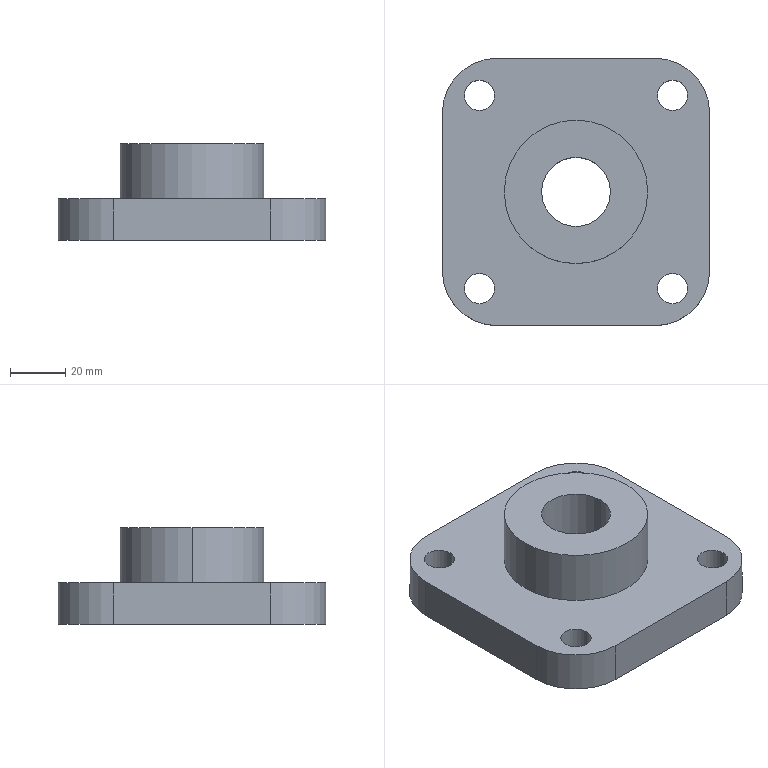Part | STEP file | Bearing housing 1 | 1 solid | 23 faces | box 97 x 97 x 35 mm | volume 155576 mm3 | cylinder 16 | plane 7 | commonest cylinder face diameters 11 x8 40 x4 25 x2 52 x2
STEP:
#1=CARTESIAN_POINT('',(28.236,16.5,35.));
#2=VERTEX_POINT('',#1);
#3=CARTESIAN_POINT('',(3.236,16.5,35.));
#4=VERTEX_POINT('',#3);
#5=CARTESIAN_POINT('',(15.736,16.5,35.));
#6=DIRECTION('',(0.,0.,-1.));
#7=DIRECTION('',(-1.,0.,0.));
#8=AXIS2_PLACEMENT_3D('',#5,#6,#7);
#9=CIRCLE('',#8,12.5);
#10=EDGE_CURVE('',#2,#4,#9,.T.);
#11=ORIENTED_EDGE('',*,*,#10,.F.);
#12=CARTESIAN_POINT('',(28.236,16.5,0.));
#13=VERTEX_POINT('',#12);
#14=CARTESIAN_POINT('',(28.236,16.5,15.));
#15=DIRECTION('',(0.,0.,-1.));
#16=VECTOR('',#15,1000.);
#17=LINE('',#14,#16);
#18=EDGE_CURVE('',#2,#13,#17,.T.);
#19=ORIENTED_EDGE('',*,*,#18,.T.);
#20=CARTESIAN_POINT('',(3.236,16.5,0.));
#21=VERTEX_POINT('',#20);
#22=CARTESIAN_POINT('',(15.736,16.5,0.));
#23=DIRECTION('',(0.,0.,-1.));
#24=DIRECTION('',(-1.,0.,0.));
#25=AXIS2_PLACEMENT_3D('',#22,#23,#24);
#26=CIRCLE('',#25,12.5);
#27=EDGE_CURVE('',#13,#21,#26,.T.);
#28=ORIENTED_EDGE('',*,*,#27,.T.);
#29=CARTESIAN_POINT('',(3.236,16.5,15.));
#30=DIRECTION('',(0.,0.,-1.));
#31=VECTOR('',#30,1000.);
#32=LINE('',#29,#31);
#33=EDGE_CURVE('',#4,#21,#32,.T.);
#34=ORIENTED_EDGE('',*,*,#33,.F.);
#35=EDGE_LOOP('',(#11,#19,#28,#34));
#36=FACE_OUTER_BOUND('',#35,.T.);
#37=CARTESIAN_POINT('',(15.736,16.5,15.));
#38=DIRECTION('',(0.,0.,-1.));
#39=DIRECTION('',(-1.,0.,0.));
#40=AXIS2_PLACEMENT_3D('',#37,#38,#39);
#41=CYLINDRICAL_SURFACE('',#40,12.5);
#42=ADVANCED_FACE('',(#36),#41,.F.);
#43=CARTESIAN_POINT('',(56.236,-18.5,15.));
#44=VERTEX_POINT('',#43);
#45=CARTESIAN_POINT('',(45.236,-18.5,15.));
#46=VERTEX_POINT('',#45);
#47=CARTESIAN_POINT('',(50.736,-18.5,15.));
#48=DIRECTION('',(0.,0.,-1.));
#49=DIRECTION('',(-1.,0.,0.));
#50=AXIS2_PLACEMENT_3D('',#47,#48,#49);
#51=CIRCLE('',#50,5.5);
#52=EDGE_CURVE('',#44,#46,#51,.T.);
#53=ORIENTED_EDGE('',*,*,#52,.F.);
#54=CARTESIAN_POINT('',(56.236,-18.5,0.));
#55=VERTEX_POINT('',#54);
#56=CARTESIAN_POINT('',(56.236,-18.5,15.));
#57=DIRECTION('',(0.,0.,-1.));
#58=VECTOR('',#57,1000.);
#59=LINE('',#56,#58);
#60=EDGE_CURVE('',#44,#55,#59,.T.);
#61=ORIENTED_EDGE('',*,*,#60,.T.);
#62=CARTESIAN_POINT('',(45.236,-18.5,0.));
#63=VERTEX_POINT('',#62);
#64=CARTESIAN_POINT('',(50.736,-18.5,0.));
#65=DIRECTION('',(0.,0.,-1.));
#66=DIRECTION('',(-1.,0.,0.));
#67=AXIS2_PLACEMENT_3D('',#64,#65,#66);
#68=CIRCLE('',#67,5.5);
#69=EDGE_CURVE('',#55,#63,#68,.T.);
#70=ORIENTED_EDGE('',*,*,#69,.T.);
#71=CARTESIAN_POINT('',(45.236,-18.5,15.));
#72=DIRECTION('',(0.,0.,-1.));
#73=VECTOR('',#72,1000.);
#74=LINE('',#71,#73);
#75=EDGE_CURVE('',#46,#63,#74,.T.);
#76=ORIENTED_EDGE('',*,*,#75,.F.);
#77=EDGE_LOOP('',(#53,#61,#70,#76));
#78=FACE_OUTER_BOUND('',#77,.T.);
#79=CARTESIAN_POINT('',(50.736,-18.5,15.));
#80=DIRECTION('',(0.,0.,-1.));
#81=DIRECTION('',(-1.,0.,0.));
#82=AXIS2_PLACEMENT_3D('',#79,#80,#81);
#83=CYLINDRICAL_SURFACE('',#82,5.5);
#84=ADVANCED_FACE('',(#78),#83,.F.);
#85=CARTESIAN_POINT('',(-13.764,51.5,15.));
#86=VERTEX_POINT('',#85);
#87=CARTESIAN_POINT('',(-24.764,51.5,15.));
#88=VERTEX_POINT('',#87);
#89=CARTESIAN_POINT('',(-19.264,51.5,15.));
#90=DIRECTION('',(0.,0.,-1.));
#91=DIRECTION('',(-1.,0.,0.));
#92=AXIS2_PLACEMENT_3D('',#89,#90,#91);
#93=CIRCLE('',#92,5.5);
#94=EDGE_CURVE('',#86,#88,#93,.T.);
#95=ORIENTED_EDGE('',*,*,#94,.F.);
#96=CARTESIAN_POINT('',(-13.764,51.5,0.));
#97=VERTEX_POINT('',#96);
#98=CARTESIAN_POINT('',(-13.764,51.5,15.));
#99=DIRECTION('',(0.,0.,-1.));
#100=VECTOR('',#99,1000.);
#101=LINE('',#98,#100);
#102=EDGE_CURVE('',#86,#97,#101,.T.);
#103=ORIENTED_EDGE('',*,*,#102,.T.);
#104=CARTESIAN_POINT('',(-24.764,51.5,0.));
#105=VERTEX_POINT('',#104);
#106=CARTESIAN_POINT('',(-19.264,51.5,0.));
#107=DIRECTION('',(0.,0.,-1.));
#108=DIRECTION('',(-1.,0.,0.));
#109=AXIS2_PLACEMENT_3D('',#106,#107,#108);
#110=CIRCLE('',#109,5.5);
#111=EDGE_CURVE('',#97,#105,#110,.T.);
#112=ORIENTED_EDGE('',*,*,#111,.T.);
#113=CARTESIAN_POINT('',(-24.764,51.5,15.));
#114=DIRECTION('',(0.,0.,-1.));
#115=VECTOR('',#114,1000.);
#116=LINE('',#113,#115);
#117=EDGE_CURVE('',#88,#105,#116,.T.);
#118=ORIENTED_EDGE('',*,*,#117,.F.);
#119=EDGE_LOOP('',(#95,#103,#112,#118));
#120=FACE_OUTER_BOUND('',#119,.T.);
#121=CARTESIAN_POINT('',(-19.264,51.5,15.));
#122=DIRECTION('',(0.,0.,-1.));
#123=DIRECTION('',(-1.,0.,0.));
#124=AXIS2_PLACEMENT_3D('',#121,#122,#123);
#125=CYLINDRICAL_SURFACE('',#124,5.5);
#126=ADVANCED_FACE('',(#120),#125,.F.);
#127=CARTESIAN_POINT('',(56.236,51.5,15.));
#128=VERTEX_POINT('',#127);
#129=CARTESIAN_POINT('',(45.236,51.5,15.));
#130=VERTEX_POINT('',#129);
#131=CARTESIAN_POINT('',(50.736,51.5,15.));
#132=DIRECTION('',(0.,0.,-1.));
#133=DIRECTION('',(-1.,0.,0.));
#134=AXIS2_PLACEMENT_3D('',#131,#132,#133);
#135=CIRCLE('',#134,5.5);
#136=EDGE_CURVE('',#128,#130,#135,.T.);
#137=ORIENTED_EDGE('',*,*,#136,.F.);
#138=CARTESIAN_POINT('',(56.236,51.5,0.));
#139=VERTEX_POINT('',#138);
#140=CARTESIAN_POINT('',(56.236,51.5,15.));
#141=DIRECTION('',(0.,0.,-1.));
#142=VECTOR('',#141,1000.);
#143=LINE('',#140,#142);
#144=EDGE_CURVE('',#128,#139,#143,.T.);
#145=ORIENTED_EDGE('',*,*,#144,.T.);
#146=CARTESIAN_POINT('',(45.236,51.5,0.));
#147=VERTEX_POINT('',#146);
#148=CARTESIAN_POINT('',(50.736,51.5,0.));
#149=DIRECTION('',(0.,0.,-1.));
#150=DIRECTION('',(-1.,0.,0.));
#151=AXIS2_PLACEMENT_3D('',#148,#149,#150);
#152=CIRCLE('',#151,5.5);
#153=EDGE_CURVE('',#139,#147,#152,.T.);
#154=ORIENTED_EDGE('',*,*,#153,.T.);
#155=CARTESIAN_POINT('',(45.236,51.5,15.));
#156=DIRECTION('',(0.,0.,-1.));
#157=VECTOR('',#156,1000.);
#158=LINE('',#155,#157);
#159=EDGE_CURVE('',#130,#147,#158,.T.);
#160=ORIENTED_EDGE('',*,*,#159,.F.);
#161=EDGE_LOOP('',(#137,#145,#154,#160));
#162=FACE_OUTER_BOUND('',#161,.T.);
#163=CARTESIAN_POINT('',(50.736,51.5,15.));
#164=DIRECTION('',(0.,0.,-1.));
#165=DIRECTION('',(-1.,0.,0.));
#166=AXIS2_PLACEMENT_3D('',#163,#164,#165);
#167=CYLINDRICAL_SURFACE('',#166,5.5);
#168=ADVANCED_FACE('',(#162),#167,.F.);
#169=CARTESIAN_POINT('',(-13.764,-18.5,15.));
#170=VERTEX_POINT('',#169);
#171=CARTESIAN_POINT('',(-24.764,-18.5,15.));
#172=VERTEX_POINT('',#171);
#173=CARTESIAN_POINT('',(-19.264,-18.5,15.));
#174=DIRECTION('',(0.,0.,-1.));
#175=DIRECTION('',(-1.,0.,0.));
#176=AXIS2_PLACEMENT_3D('',#173,#174,#175);
#177=CIRCLE('',#176,5.5);
#178=EDGE_CURVE('',#170,#172,#177,.T.);
#179=ORIENTED_EDGE('',*,*,#178,.F.);
#180=CARTESIAN_POINT('',(-13.764,-18.5,0.));
#181=VERTEX_POINT('',#180);
#182=CARTESIAN_POINT('',(-13.764,-18.5,15.));
#183=DIRECTION('',(0.,0.,-1.));
#184=VECTOR('',#183,1000.);
#185=LINE('',#182,#184);
#186=EDGE_CURVE('',#170,#181,#185,.T.);
#187=ORIENTED_EDGE('',*,*,#186,.T.);
#188=CARTESIAN_POINT('',(-24.764,-18.5,0.));
#189=VERTEX_POINT('',#188);
#190=CARTESIAN_POINT('',(-19.264,-18.5,0.));
#191=DIRECTION('',(0.,0.,-1.));
#192=DIRECTION('',(-1.,0.,0.));
#193=AXIS2_PLACEMENT_3D('',#190,#191,#192);
#194=CIRCLE('',#193,5.5);
#195=EDGE_CURVE('',#181,#189,#194,.T.);
#196=ORIENTED_EDGE('',*,*,#195,.T.);
#197=CARTESIAN_POINT('',(-24.764,-18.5,15.));
#198=DIRECTION('',(0.,0.,-1.));
#199=VECTOR('',#198,1000.);
#200=LINE('',#197,#199);
#201=EDGE_CURVE('',#172,#189,#200,.T.);
#202=ORIENTED_EDGE('',*,*,#201,.F.);
#203=EDGE_LOOP('',(#179,#187,#196,#202));
#204=FACE_OUTER_BOUND('',#203,.T.);
#205=CARTESIAN_POINT('',(-19.264,-18.5,15.));
#206=DIRECTION('',(0.,0.,-1.));
#207=DIRECTION('',(-1.,0.,0.));
#208=AXIS2_PLACEMENT_3D('',#205,#206,#207);
#209=CYLINDRICAL_SURFACE('',#208,5.5);
#210=ADVANCED_FACE('',(#204),#209,.F.);
#211=CARTESIAN_POINT('',(41.736,16.5,35.));
#212=VERTEX_POINT('',#211);
#213=CARTESIAN_POINT('',(-10.264,16.5,35.));
#214=VERTEX_POINT('',#213);
#215=CARTESIAN_POINT('',(15.736,16.5,35.));
#216=DIRECTION('',(0.,0.,1.));
#217=DIRECTION('',(-1.,0.,0.));
#218=AXIS2_PLACEMENT_3D('',#215,#216,#217);
#219=CIRCLE('',#218,26.);
#220=EDGE_CURVE('',#212,#214,#219,.T.);
#221=ORIENTED_EDGE('',*,*,#220,.F.);
#222=CARTESIAN_POINT('',(41.736,16.5,15.));
#223=VERTEX_POINT('',#222);
#224=CARTESIAN_POINT('',(41.736,16.5,35.));
#225=DIRECTION('',(0.,0.,-1.));
#226=VECTOR('',#225,1000.);
#227=LINE('',#224,#226);
#228=EDGE_CURVE('',#212,#223,#227,.T.);
#229=ORIENTED_EDGE('',*,*,#228,.T.);
#230=CARTESIAN_POINT('',(-10.264,16.5,15.));
#231=VERTEX_POINT('',#230);
#232=CARTESIAN_POINT('',(15.736,16.5,15.));
#233=DIRECTION('',(0.,0.,-1.));
#234=DIRECTION('',(-1.,0.,0.));
#235=AXIS2_PLACEMENT_3D('',#232,#233,#234);
#236=CIRCLE('',#235,26.);
#237=EDGE_CURVE('',#231,#223,#236,.T.);
#238=ORIENTED_EDGE('',*,*,#237,.F.);
#239=CARTESIAN_POINT('',(-10.264,16.5,35.));
#240=DIRECTION('',(0.,0.,-1.));
#241=VECTOR('',#240,1000.);
#242=LINE('',#239,#241);
#243=EDGE_CURVE('',#214,#231,#242,.T.);
#244=ORIENTED_EDGE('',*,*,#243,.F.);
#245=EDGE_LOOP('',(#221,#229,#238,#244));
#246=FACE_OUTER_BOUND('',#245,.T.);
#247=CARTESIAN_POINT('',(15.736,16.5,35.));
#248=DIRECTION('',(0.,0.,-1.));
#249=DIRECTION('',(-1.,0.,0.));
#250=AXIS2_PLACEMENT_3D('',#247,#248,#249);
#251=CYLINDRICAL_SURFACE('',#250,26.);
#252=ADVANCED_FACE('',(#246),#251,.T.);
#253=CARTESIAN_POINT('',(15.736,16.5,0.));
#254=DIRECTION('',(0.,0.,-1.));
#255=DIRECTION('',(-1.,0.,0.));
#256=AXIS2_PLACEMENT_3D('',#253,#254,#255);
#257=CIRCLE('',#256,12.5);
#258=EDGE_CURVE('',#21,#13,#257,.T.);
#259=ORIENTED_EDGE('',*,*,#258,.F.);
#260=ORIENTED_EDGE('',*,*,#27,.F.);
#261=EDGE_LOOP('',(#259,#260));
#262=FACE_BOUND('',#261,.T.);
#263=CARTESIAN_POINT('',(50.736,-18.5,0.));
#264=DIRECTION('',(0.,0.,-1.));
#265=DIRECTION('',(-1.,0.,0.));
#266=AXIS2_PLACEMENT_3D('',#263,#264,#265);
#267=CIRCLE('',#266,5.5);
#268=EDGE_CURVE('',#63,#55,#267,.T.);
#269=ORIENTED_EDGE('',*,*,#268,.F.);
#270=ORIENTED_EDGE('',*,*,#69,.F.);
#271=EDGE_LOOP('',(#269,#270));
#272=FACE_BOUND('',#271,.T.);
#273=CARTESIAN_POINT('',(-19.264,51.5,0.));
#274=DIRECTION('',(0.,0.,-1.));
#275=DIRECTION('',(-1.,0.,0.));
#276=AXIS2_PLACEMENT_3D('',#273,#274,#275);
#277=CIRCLE('',#276,5.5);
#278=EDGE_CURVE('',#105,#97,#277,.T.);
#279=ORIENTED_EDGE('',*,*,#278,.F.);
#280=ORIENTED_EDGE('',*,*,#111,.F.);
#281=EDGE_LOOP('',(#279,#280));
#282=FACE_BOUND('',#281,.T.);
#283=CARTESIAN_POINT('',(-32.764,-12.,0.));
#284=VERTEX_POINT('',#283);
#285=CARTESIAN_POINT('',(-12.764,-32.,0.));
#286=VERTEX_POINT('',#285);
#287=CARTESIAN_POINT('',(-12.764,-12.,0.));
#288=DIRECTION('',(0.,0.,1.));
#289=DIRECTION('',(-1.,0.,0.));
#290=AXIS2_PLACEMENT_3D('',#287,#288,#289);
#291=CIRCLE('',#290,20.);
#292=EDGE_CURVE('',#284,#286,#291,.T.);
#293=ORIENTED_EDGE('',*,*,#292,.F.);
#294=CARTESIAN_POINT('',(-32.764,45.,0.));
#295=VERTEX_POINT('',#294);
#296=CARTESIAN_POINT('',(-32.764,65.,0.));
#297=DIRECTION('',(0.,-1.,0.));
#298=VECTOR('',#297,1000.);
#299=LINE('',#296,#298);
#300=EDGE_CURVE('',#295,#284,#299,.T.);
#301=ORIENTED_EDGE('',*,*,#300,.F.);
#302=CARTESIAN_POINT('',(-12.764,65.,0.));
#303=VERTEX_POINT('',#302);
#304=CARTESIAN_POINT('',(-12.764,45.,0.));
#305=DIRECTION('',(0.,0.,1.));
#306=DIRECTION('',(-1.,0.,0.));
#307=AXIS2_PLACEMENT_3D('',#304,#305,#306);
#308=CIRCLE('',#307,20.);
#309=EDGE_CURVE('',#303,#295,#308,.T.);
#310=ORIENTED_EDGE('',*,*,#309,.F.);
#311=CARTESIAN_POINT('',(44.236,65.,0.));
#312=VERTEX_POINT('',#311);
#313=CARTESIAN_POINT('',(-32.764,65.,0.));
#314=DIRECTION('',(-1.,0.,0.));
#315=VECTOR('',#314,1000.);
#316=LINE('',#313,#315);
#317=EDGE_CURVE('',#312,#303,#316,.T.);
#318=ORIENTED_EDGE('',*,*,#317,.F.);
#319=CARTESIAN_POINT('',(64.236,45.,0.));
#320=VERTEX_POINT('',#319);
#321=CARTESIAN_POINT('',(44.236,45.,0.));
#322=DIRECTION('',(0.,0.,1.));
#323=DIRECTION('',(-1.,0.,0.));
#324=AXIS2_PLACEMENT_3D('',#321,#322,#323);
#325=CIRCLE('',#324,20.);
#326=EDGE_CURVE('',#320,#312,#325,.T.);
#327=ORIENTED_EDGE('',*,*,#326,.F.);
#328=CARTESIAN_POINT('',(64.236,-12.,0.));
#329=VERTEX_POINT('',#328);
#330=CARTESIAN_POINT('',(64.236,65.,0.));
#331=DIRECTION('',(0.,1.,0.));
#332=VECTOR('',#331,1000.);
#333=LINE('',#330,#332);
#334=EDGE_CURVE('',#329,#320,#333,.T.);
#335=ORIENTED_EDGE('',*,*,#334,.F.);
#336=CARTESIAN_POINT('',(44.236,-32.,0.));
#337=VERTEX_POINT('',#336);
#338=CARTESIAN_POINT('',(44.236,-12.,0.));
#339=DIRECTION('',(0.,0.,1.));
#340=DIRECTION('',(-1.,0.,0.));
#341=AXIS2_PLACEMENT_3D('',#338,#339,#340);
#342=CIRCLE('',#341,20.);
#343=EDGE_CURVE('',#337,#329,#342,.T.);
#344=ORIENTED_EDGE('',*,*,#343,.F.);
#345=CARTESIAN_POINT('',(-32.764,-32.,0.));
#346=DIRECTION('',(1.,0.,0.));
#347=VECTOR('',#346,1000.);
#348=LINE('',#345,#347);
#349=EDGE_CURVE('',#286,#337,#348,.T.);
#350=ORIENTED_EDGE('',*,*,#349,.F.);
#351=EDGE_LOOP('',(#293,#301,#310,#318,#327,#335,#344,#350));
#352=FACE_OUTER_BOUND('',#351,.T.);
#353=CARTESIAN_POINT('',(50.736,51.5,0.));
#354=DIRECTION('',(0.,0.,-1.));
#355=DIRECTION('',(-1.,0.,0.));
#356=AXIS2_PLACEMENT_3D('',#353,#354,#355);
#357=CIRCLE('',#356,5.5);
#358=EDGE_CURVE('',#147,#139,#357,.T.);
#359=ORIENTED_EDGE('',*,*,#358,.F.);
#360=ORIENTED_EDGE('',*,*,#153,.F.);
#361=EDGE_LOOP('',(#359,#360));
#362=FACE_BOUND('',#361,.T.);
#363=CARTESIAN_POINT('',(-19.264,-18.5,0.));
#364=DIRECTION('',(0.,0.,-1.));
#365=DIRECTION('',(-1.,0.,0.));
#366=AXIS2_PLACEMENT_3D('',#363,#364,#365);
#367=CIRCLE('',#366,5.5);
#368=EDGE_CURVE('',#189,#181,#367,.T.);
#369=ORIENTED_EDGE('',*,*,#368,.F.);
#370=ORIENTED_EDGE('',*,*,#195,.F.);
#371=EDGE_LOOP('',(#369,#370));
#372=FACE_BOUND('',#371,.T.);
#373=CARTESIAN_POINT('',(-32.764,65.,0.));
#374=DIRECTION('',(0.,0.,1.));
#375=DIRECTION('',(1.,0.,0.));
#376=AXIS2_PLACEMENT_3D('',#373,#374,#375);
#377=PLANE('',#376);
#378=ADVANCED_FACE('',(#262,#272,#282,#352,#362,#372),#377,.F.);
#379=ORIENTED_EDGE('',*,*,#18,.F.);
#380=CARTESIAN_POINT('',(15.736,16.5,35.));
#381=DIRECTION('',(0.,0.,-1.));
#382=DIRECTION('',(-1.,0.,0.));
#383=AXIS2_PLACEMENT_3D('',#380,#381,#382);
#384=CIRCLE('',#383,12.5);
#385=EDGE_CURVE('',#4,#2,#384,.T.);
#386=ORIENTED_EDGE('',*,*,#385,.F.);
#387=ORIENTED_EDGE('',*,*,#33,.T.);
#388=ORIENTED_EDGE('',*,*,#258,.T.);
#389=EDGE_LOOP('',(#379,#386,#387,#388));
#390=FACE_OUTER_BOUND('',#389,.T.);
#391=CARTESIAN_POINT('',(15.736,16.5,15.));
#392=DIRECTION('',(0.,0.,-1.));
#393=DIRECTION('',(-1.,0.,0.));
#394=AXIS2_PLACEMENT_3D('',#391,#392,#393);
#395=CYLINDRICAL_SURFACE('',#394,12.5);
#396=ADVANCED_FACE('',(#390),#395,.F.);
#397=ORIENTED_EDGE('',*,*,#60,.F.);
#398=CARTESIAN_POINT('',(50.736,-18.5,15.));
#399=DIRECTION('',(0.,0.,-1.));
#400=DIRECTION('',(-1.,0.,0.));
#401=AXIS2_PLACEMENT_3D('',#398,#399,#400);
#402=CIRCLE('',#401,5.5);
#403=EDGE_CURVE('',#46,#44,#402,.T.);
#404=ORIENTED_EDGE('',*,*,#403,.F.);
#405=ORIENTED_EDGE('',*,*,#75,.T.);
#406=ORIENTED_EDGE('',*,*,#268,.T.);
#407=EDGE_LOOP('',(#397,#404,#405,#406));
#408=FACE_OUTER_BOUND('',#407,.T.);
#409=CARTESIAN_POINT('',(50.736,-18.5,15.));
#410=DIRECTION('',(0.,0.,-1.));
#411=DIRECTION('',(-1.,0.,0.));
#412=AXIS2_PLACEMENT_3D('',#409,#410,#411);
#413=CYLINDRICAL_SURFACE('',#412,5.5);
#414=ADVANCED_FACE('',(#408),#413,.F.);
#415=ORIENTED_EDGE('',*,*,#102,.F.);
#416=CARTESIAN_POINT('',(-19.264,51.5,15.));
#417=DIRECTION('',(0.,0.,-1.));
#418=DIRECTION('',(-1.,0.,0.));
#419=AXIS2_PLACEMENT_3D('',#416,#417,#418);
#420=CIRCLE('',#419,5.5);
#421=EDGE_CURVE('',#88,#86,#420,.T.);
#422=ORIENTED_EDGE('',*,*,#421,.F.);
#423=ORIENTED_EDGE('',*,*,#117,.T.);
#424=ORIENTED_EDGE('',*,*,#278,.T.);
#425=EDGE_LOOP('',(#415,#422,#423,#424));
#426=FACE_OUTER_BOUND('',#425,.T.);
#427=CARTESIAN_POINT('',(-19.264,51.5,15.));
#428=DIRECTION('',(0.,0.,-1.));
#429=DIRECTION('',(-1.,0.,0.));
#430=AXIS2_PLACEMENT_3D('',#427,#428,#429);
#431=CYLINDRICAL_SURFACE('',#430,5.5);
#432=ADVANCED_FACE('',(#426),#431,.F.);
#433=CARTESIAN_POINT('',(-12.764,-32.,15.));
#434=VERTEX_POINT('',#433);
#435=CARTESIAN_POINT('',(-12.764,-32.,15.));
#436=DIRECTION('',(0.,0.,1.));
#437=VECTOR('',#436,1000.);
#438=LINE('',#435,#437);
#439=EDGE_CURVE('',#286,#434,#438,.T.);
#440=ORIENTED_EDGE('',*,*,#439,.F.);
#441=ORIENTED_EDGE('',*,*,#349,.T.);
#442=CARTESIAN_POINT('',(44.236,-32.,15.));
#443=VERTEX_POINT('',#442);
#444=CARTESIAN_POINT('',(44.236,-32.,15.));
#445=DIRECTION('',(0.,0.,-1.));
#446=VECTOR('',#445,1000.);
#447=LINE('',#444,#446);
#448=EDGE_CURVE('',#443,#337,#447,.T.);
#449=ORIENTED_EDGE('',*,*,#448,.F.);
#450=CARTESIAN_POINT('',(-32.764,-32.,15.));
#451=DIRECTION('',(1.,0.,0.));
#452=VECTOR('',#451,1000.);
#453=LINE('',#450,#452);
#454=EDGE_CURVE('',#434,#443,#453,.T.);
#455=ORIENTED_EDGE('',*,*,#454,.F.);
#456=EDGE_LOOP('',(#440,#441,#449,#455));
#457=FACE_OUTER_BOUND('',#456,.T.);
#458=CARTESIAN_POINT('',(-32.764,-32.,15.));
#459=DIRECTION('',(0.,1.,0.));
#460=DIRECTION('',(0.,0.,1.));
#461=AXIS2_PLACEMENT_3D('',#458,#459,#460);
#462=PLANE('',#461);
#463=ADVANCED_FACE('',(#457),#462,.F.);
#464=ORIENTED_EDGE('',*,*,#292,.T.);
#465=ORIENTED_EDGE('',*,*,#439,.T.);
#466=CARTESIAN_POINT('',(-32.764,-12.,15.));
#467=VERTEX_POINT('',#466);
#468=CARTESIAN_POINT('',(-12.764,-12.,15.));
#469=DIRECTION('',(0.,0.,-1.));
#470=DIRECTION('',(-1.,0.,0.));
#471=AXIS2_PLACEMENT_3D('',#468,#469,#470);
#472=CIRCLE('',#471,20.);
#473=EDGE_CURVE('',#434,#467,#472,.T.);
#474=ORIENTED_EDGE('',*,*,#473,.T.);
#475=CARTESIAN_POINT('',(-32.764,-12.,15.));
#476=DIRECTION('',(0.,0.,-1.));
#477=VECTOR('',#476,1000.);
#478=LINE('',#475,#477);
#479=EDGE_CURVE('',#467,#284,#478,.T.);
#480=ORIENTED_EDGE('',*,*,#479,.T.);
#481=EDGE_LOOP('',(#464,#465,#474,#480));
#482=FACE_OUTER_BOUND('',#481,.T.);
#483=CARTESIAN_POINT('',(-12.764,-12.,15.));
#484=DIRECTION('',(0.,0.,-1.));
#485=DIRECTION('',(-1.,0.,0.));
#486=AXIS2_PLACEMENT_3D('',#483,#484,#485);
#487=CYLINDRICAL_SURFACE('',#486,20.);
#488=ADVANCED_FACE('',(#482),#487,.T.);
#489=ORIENTED_EDGE('',*,*,#479,.F.);
#490=CARTESIAN_POINT('',(-32.764,45.,15.));
#491=VERTEX_POINT('',#490);
#492=CARTESIAN_POINT('',(-32.764,65.,15.));
#493=DIRECTION('',(0.,-1.,0.));
#494=VECTOR('',#493,1000.);
#495=LINE('',#492,#494);
#496=EDGE_CURVE('',#491,#467,#495,.T.);
#497=ORIENTED_EDGE('',*,*,#496,.F.);
#498=CARTESIAN_POINT('',(-32.764,45.,15.));
#499=DIRECTION('',(0.,0.,1.));
#500=VECTOR('',#499,1000.);
#501=LINE('',#498,#500);
#502=EDGE_CURVE('',#295,#491,#501,.T.);
#503=ORIENTED_EDGE('',*,*,#502,.F.);
#504=ORIENTED_EDGE('',*,*,#300,.T.);
#505=EDGE_LOOP('',(#489,#497,#503,#504));
#506=FACE_OUTER_BOUND('',#505,.T.);
#507=CARTESIAN_POINT('',(-32.764,65.,15.));
#508=DIRECTION('',(1.,0.,0.));
#509=DIRECTION('',(0.,1.,0.));
#510=AXIS2_PLACEMENT_3D('',#507,#508,#509);
#511=PLANE('',#510);
#512=ADVANCED_FACE('',(#506),#511,.F.);
#513=ORIENTED_EDGE('',*,*,#309,.T.);
#514=ORIENTED_EDGE('',*,*,#502,.T.);
#515=CARTESIAN_POINT('',(-12.764,65.,15.));
#516=VERTEX_POINT('',#515);
#517=CARTESIAN_POINT('',(-12.764,45.,15.));
#518=DIRECTION('',(0.,0.,-1.));
#519=DIRECTION('',(-1.,0.,0.));
#520=AXIS2_PLACEMENT_3D('',#517,#518,#519);
#521=CIRCLE('',#520,20.);
#522=EDGE_CURVE('',#491,#516,#521,.T.);
#523=ORIENTED_EDGE('',*,*,#522,.T.);
#524=CARTESIAN_POINT('',(-12.764,65.,15.));
#525=DIRECTION('',(0.,0.,-1.));
#526=VECTOR('',#525,1000.);
#527=LINE('',#524,#526);
#528=EDGE_CURVE('',#516,#303,#527,.T.);
#529=ORIENTED_EDGE('',*,*,#528,.T.);
#530=EDGE_LOOP('',(#513,#514,#523,#529));
#531=FACE_OUTER_BOUND('',#530,.T.);
#532=CARTESIAN_POINT('',(-12.764,45.,15.));
#533=DIRECTION('',(0.,0.,-1.));
#534=DIRECTION('',(-1.,0.,0.));
#535=AXIS2_PLACEMENT_3D('',#532,#533,#534);
#536=CYLINDRICAL_SURFACE('',#535,20.);
#537=ADVANCED_FACE('',(#531),#536,.T.);
#538=CARTESIAN_POINT('',(44.236,65.,15.));
#539=VERTEX_POINT('',#538);
#540=CARTESIAN_POINT('',(44.236,65.,15.));
#541=DIRECTION('',(0.,0.,1.));
#542=VECTOR('',#541,1000.);
#543=LINE('',#540,#542);
#544=EDGE_CURVE('',#312,#539,#543,.T.);
#545=ORIENTED_EDGE('',*,*,#544,.F.);
#546=ORIENTED_EDGE('',*,*,#317,.T.);
#547=ORIENTED_EDGE('',*,*,#528,.F.);
#548=CARTESIAN_POINT('',(-32.764,65.,15.));
#549=DIRECTION('',(-1.,0.,0.));
#550=VECTOR('',#549,1000.);
#551=LINE('',#548,#550);
#552=EDGE_CURVE('',#539,#516,#551,.T.);
#553=ORIENTED_EDGE('',*,*,#552,.F.);
#554=EDGE_LOOP('',(#545,#546,#547,#553));
#555=FACE_OUTER_BOUND('',#554,.T.);
#556=CARTESIAN_POINT('',(-32.764,65.,15.));
#557=DIRECTION('',(0.,-1.,0.));
#558=DIRECTION('',(0.,0.,-1.));
#559=AXIS2_PLACEMENT_3D('',#556,#557,#558);
#560=PLANE('',#559);
#561=ADVANCED_FACE('',(#555),#560,.F.);
#562=ORIENTED_EDGE('',*,*,#326,.T.);
#563=ORIENTED_EDGE('',*,*,#544,.T.);
#564=CARTESIAN_POINT('',(64.236,45.,15.));
#565=VERTEX_POINT('',#564);
#566=CARTESIAN_POINT('',(44.236,45.,15.));
#567=DIRECTION('',(0.,0.,-1.));
#568=DIRECTION('',(-1.,0.,0.));
#569=AXIS2_PLACEMENT_3D('',#566,#567,#568);
#570=CIRCLE('',#569,20.);
#571=EDGE_CURVE('',#539,#565,#570,.T.);
#572=ORIENTED_EDGE('',*,*,#571,.T.);
#573=CARTESIAN_POINT('',(64.236,45.,15.));
#574=DIRECTION('',(0.,0.,-1.));
#575=VECTOR('',#574,1000.);
#576=LINE('',#573,#575);
#577=EDGE_CURVE('',#565,#320,#576,.T.);
#578=ORIENTED_EDGE('',*,*,#577,.T.);
#579=EDGE_LOOP('',(#562,#563,#572,#578));
#580=FACE_OUTER_BOUND('',#579,.T.);
#581=CARTESIAN_POINT('',(44.236,45.,15.));
#582=DIRECTION('',(0.,0.,-1.));
#583=DIRECTION('',(-1.,0.,0.));
#584=AXIS2_PLACEMENT_3D('',#581,#582,#583);
#585=CYLINDRICAL_SURFACE('',#584,20.);
#586=ADVANCED_FACE('',(#580),#585,.T.);
#587=CARTESIAN_POINT('',(64.236,-12.,15.));
#588=VERTEX_POINT('',#587);
#589=CARTESIAN_POINT('',(64.236,-12.,15.));
#590=DIRECTION('',(0.,0.,1.));
#591=VECTOR('',#590,1000.);
#592=LINE('',#589,#591);
#593=EDGE_CURVE('',#329,#588,#592,.T.);
#594=ORIENTED_EDGE('',*,*,#593,.F.);
#595=ORIENTED_EDGE('',*,*,#334,.T.);
#596=ORIENTED_EDGE('',*,*,#577,.F.);
#597=CARTESIAN_POINT('',(64.236,65.,15.));
#598=DIRECTION('',(0.,1.,0.));
#599=VECTOR('',#598,1000.);
#600=LINE('',#597,#599);
#601=EDGE_CURVE('',#588,#565,#600,.T.);
#602=ORIENTED_EDGE('',*,*,#601,.F.);
#603=EDGE_LOOP('',(#594,#595,#596,#602));
#604=FACE_OUTER_BOUND('',#603,.T.);
#605=CARTESIAN_POINT('',(64.236,65.,15.));
#606=DIRECTION('',(-1.,0.,0.));
#607=DIRECTION('',(0.,0.,1.));
#608=AXIS2_PLACEMENT_3D('',#605,#606,#607);
#609=PLANE('',#608);
#610=ADVANCED_FACE('',(#604),#609,.F.);
#611=ORIENTED_EDGE('',*,*,#343,.T.);
#612=ORIENTED_EDGE('',*,*,#593,.T.);
#613=CARTESIAN_POINT('',(44.236,-12.,15.));
#614=DIRECTION('',(0.,0.,-1.));
#615=DIRECTION('',(-1.,0.,0.));
#616=AXIS2_PLACEMENT_3D('',#613,#614,#615);
#617=CIRCLE('',#616,20.);
#618=EDGE_CURVE('',#588,#443,#617,.T.);
#619=ORIENTED_EDGE('',*,*,#618,.T.);
#620=ORIENTED_EDGE('',*,*,#448,.T.);
#621=EDGE_LOOP('',(#611,#612,#619,#620));
#622=FACE_OUTER_BOUND('',#621,.T.);
#623=CARTESIAN_POINT('',(44.236,-12.,15.));
#624=DIRECTION('',(0.,0.,-1.));
#625=DIRECTION('',(-1.,0.,0.));
#626=AXIS2_PLACEMENT_3D('',#623,#624,#625);
#627=CYLINDRICAL_SURFACE('',#626,20.);
#628=ADVANCED_FACE('',(#622),#627,.T.);
#629=ORIENTED_EDGE('',*,*,#144,.F.);
#630=CARTESIAN_POINT('',(50.736,51.5,15.));
#631=DIRECTION('',(0.,0.,-1.));
#632=DIRECTION('',(-1.,0.,0.));
#633=AXIS2_PLACEMENT_3D('',#630,#631,#632);
#634=CIRCLE('',#633,5.5);
#635=EDGE_CURVE('',#130,#128,#634,.T.);
#636=ORIENTED_EDGE('',*,*,#635,.F.);
#637=ORIENTED_EDGE('',*,*,#159,.T.);
#638=ORIENTED_EDGE('',*,*,#358,.T.);
#639=EDGE_LOOP('',(#629,#636,#637,#638));
#640=FACE_OUTER_BOUND('',#639,.T.);
#641=CARTESIAN_POINT('',(50.736,51.5,15.));
#642=DIRECTION('',(0.,0.,-1.));
#643=DIRECTION('',(-1.,0.,0.));
#644=AXIS2_PLACEMENT_3D('',#641,#642,#643);
#645=CYLINDRICAL_SURFACE('',#644,5.5);
#646=ADVANCED_FACE('',(#640),#645,.F.);
#647=ORIENTED_EDGE('',*,*,#186,.F.);
#648=CARTESIAN_POINT('',(-19.264,-18.5,15.));
#649=DIRECTION('',(0.,0.,-1.));
#650=DIRECTION('',(-1.,0.,0.));
#651=AXIS2_PLACEMENT_3D('',#648,#649,#650);
#652=CIRCLE('',#651,5.5);
#653=EDGE_CURVE('',#172,#170,#652,.T.);
#654=ORIENTED_EDGE('',*,*,#653,.F.);
#655=ORIENTED_EDGE('',*,*,#201,.T.);
#656=ORIENTED_EDGE('',*,*,#368,.T.);
#657=EDGE_LOOP('',(#647,#654,#655,#656));
#658=FACE_OUTER_BOUND('',#657,.T.);
#659=CARTESIAN_POINT('',(-19.264,-18.5,15.));
#660=DIRECTION('',(0.,0.,-1.));
#661=DIRECTION('',(-1.,0.,0.));
#662=AXIS2_PLACEMENT_3D('',#659,#660,#661);
#663=CYLINDRICAL_SURFACE('',#662,5.5);
#664=ADVANCED_FACE('',(#658),#663,.F.);
#665=ORIENTED_EDGE('',*,*,#385,.T.);
#666=ORIENTED_EDGE('',*,*,#10,.T.);
#667=EDGE_LOOP('',(#665,#666));
#668=FACE_BOUND('',#667,.T.);
#669=CARTESIAN_POINT('',(15.736,16.5,35.));
#670=DIRECTION('',(0.,0.,1.));
#671=DIRECTION('',(-1.,0.,0.));
#672=AXIS2_PLACEMENT_3D('',#669,#670,#671);
#673=CIRCLE('',#672,26.);
#674=EDGE_CURVE('',#214,#212,#673,.T.);
#675=ORIENTED_EDGE('',*,*,#674,.T.);
#676=ORIENTED_EDGE('',*,*,#220,.T.);
#677=EDGE_LOOP('',(#675,#676));
#678=FACE_OUTER_BOUND('',#677,.T.);
#679=CARTESIAN_POINT('',(15.736,16.5,35.));
#680=DIRECTION('',(0.,0.,1.));
#681=DIRECTION('',(1.,0.,0.));
#682=AXIS2_PLACEMENT_3D('',#679,#680,#681);
#683=PLANE('',#682);
#684=ADVANCED_FACE('',(#668,#678),#683,.T.);
#685=ORIENTED_EDGE('',*,*,#237,.T.);
#686=CARTESIAN_POINT('',(15.736,16.5,15.));
#687=DIRECTION('',(0.,0.,-1.));
#688=DIRECTION('',(-1.,0.,0.));
#689=AXIS2_PLACEMENT_3D('',#686,#687,#688);
#690=CIRCLE('',#689,26.);
#691=EDGE_CURVE('',#223,#231,#690,.T.);
#692=ORIENTED_EDGE('',*,*,#691,.T.);
#693=EDGE_LOOP('',(#685,#692));
#694=FACE_BOUND('',#693,.T.);
#695=ORIENTED_EDGE('',*,*,#653,.T.);
#696=ORIENTED_EDGE('',*,*,#178,.T.);
#697=EDGE_LOOP('',(#695,#696));
#698=FACE_BOUND('',#697,.T.);
#699=ORIENTED_EDGE('',*,*,#635,.T.);
#700=ORIENTED_EDGE('',*,*,#136,.T.);
#701=EDGE_LOOP('',(#699,#700));
#702=FACE_BOUND('',#701,.T.);
#703=ORIENTED_EDGE('',*,*,#552,.T.);
#704=ORIENTED_EDGE('',*,*,#522,.F.);
#705=ORIENTED_EDGE('',*,*,#496,.T.);
#706=ORIENTED_EDGE('',*,*,#473,.F.);
#707=ORIENTED_EDGE('',*,*,#454,.T.);
#708=ORIENTED_EDGE('',*,*,#618,.F.);
#709=ORIENTED_EDGE('',*,*,#601,.T.);
#710=ORIENTED_EDGE('',*,*,#571,.F.);
#711=EDGE_LOOP('',(#703,#704,#705,#706,#707,#708,#709,#710));
#712=FACE_OUTER_BOUND('',#711,.T.);
#713=ORIENTED_EDGE('',*,*,#421,.T.);
#714=ORIENTED_EDGE('',*,*,#94,.T.);
#715=EDGE_LOOP('',(#713,#714));
#716=FACE_BOUND('',#715,.T.);
#717=ORIENTED_EDGE('',*,*,#403,.T.);
#718=ORIENTED_EDGE('',*,*,#52,.T.);
#719=EDGE_LOOP('',(#717,#718));
#720=FACE_BOUND('',#719,.T.);
#721=CARTESIAN_POINT('',(-32.764,65.,15.));
#722=DIRECTION('',(0.,0.,1.));
#723=DIRECTION('',(1.,0.,0.));
#724=AXIS2_PLACEMENT_3D('',#721,#722,#723);
#725=PLANE('',#724);
#726=ADVANCED_FACE('',(#694,#698,#702,#712,#716,#720),#725,.T.);
#727=ORIENTED_EDGE('',*,*,#228,.F.);
#728=ORIENTED_EDGE('',*,*,#674,.F.);
#729=ORIENTED_EDGE('',*,*,#243,.T.);
#730=ORIENTED_EDGE('',*,*,#691,.F.);
#731=EDGE_LOOP('',(#727,#728,#729,#730));
#732=FACE_OUTER_BOUND('',#731,.T.);
#733=CARTESIAN_POINT('',(15.736,16.5,35.));
#734=DIRECTION('',(0.,0.,-1.));
#735=DIRECTION('',(-1.,0.,0.));
#736=AXIS2_PLACEMENT_3D('',#733,#734,#735);
#737=CYLINDRICAL_SURFACE('',#736,26.);
#738=ADVANCED_FACE('',(#732),#737,.T.);
#739=CLOSED_SHELL('',(#42,#84,#126,#168,#210,#252,#378,#396,#414,#432,#463,#488,#512,#537,#561,#586,#610,#628,#646,#664,#684,#726,#738));
#740=MANIFOLD_SOLID_BREP('',#739);
#741=CARTESIAN_POINT('',(0.,0.,0.));
#742=DIRECTION('',(0.,0.,1.));
#743=DIRECTION('',(1.,0.,0.));
#744=AXIS2_PLACEMENT_3D('',#741,#742,#743);
#745=(LENGTH_UNIT()NAMED_UNIT(*)SI_UNIT(.MILLI.,.METRE.));
#746=UNCERTAINTY_MEASURE_WITH_UNIT(LENGTH_MEASURE(0.00001),#745,'','');
#747=(NAMED_UNIT(*)PLANE_ANGLE_UNIT()SI_UNIT($,.RADIAN.));
#748=(NAMED_UNIT(*)SI_UNIT($,.STERADIAN.)SOLID_ANGLE_UNIT());
#749=(GEOMETRIC_REPRESENTATION_CONTEXT(3)GLOBAL_UNCERTAINTY_ASSIGNED_CONTEXT((#746))GLOBAL_UNIT_ASSIGNED_CONTEXT((#745,#747,#748))REPRESENTATION_CONTEXT('',''));
#750=ADVANCED_BREP_SHAPE_REPRESENTATION('',(#740,#744),#749);